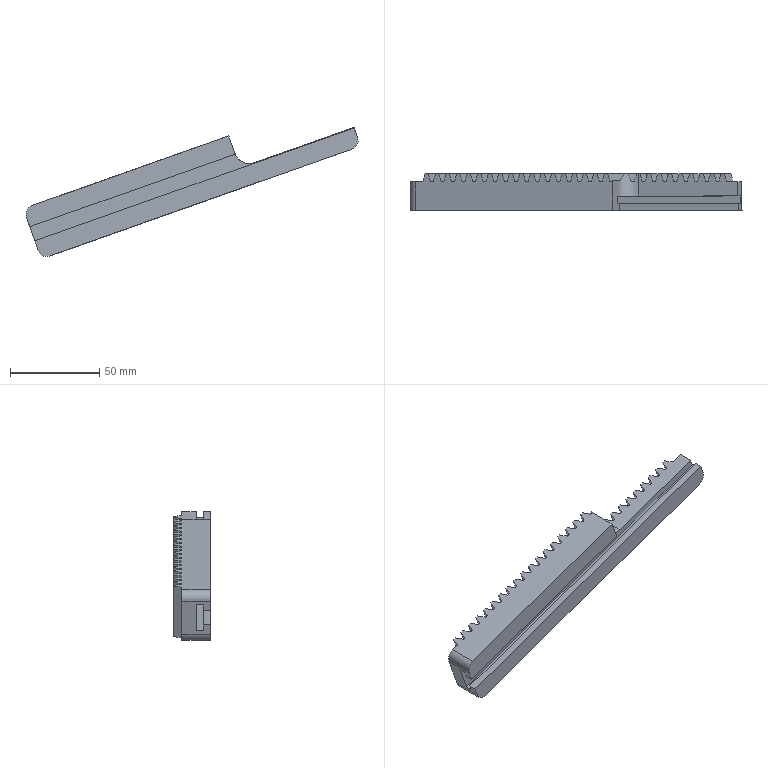Part | STEP file | RACK1_id410_x_t | 1 solid | 189 faces | box 186.352 x 20.596 x 72.41 mm | volume 67641 mm3 | plane 128 | cylinder 61 | commonest cylinder face diameters 1 x56 10 x3 17 x2